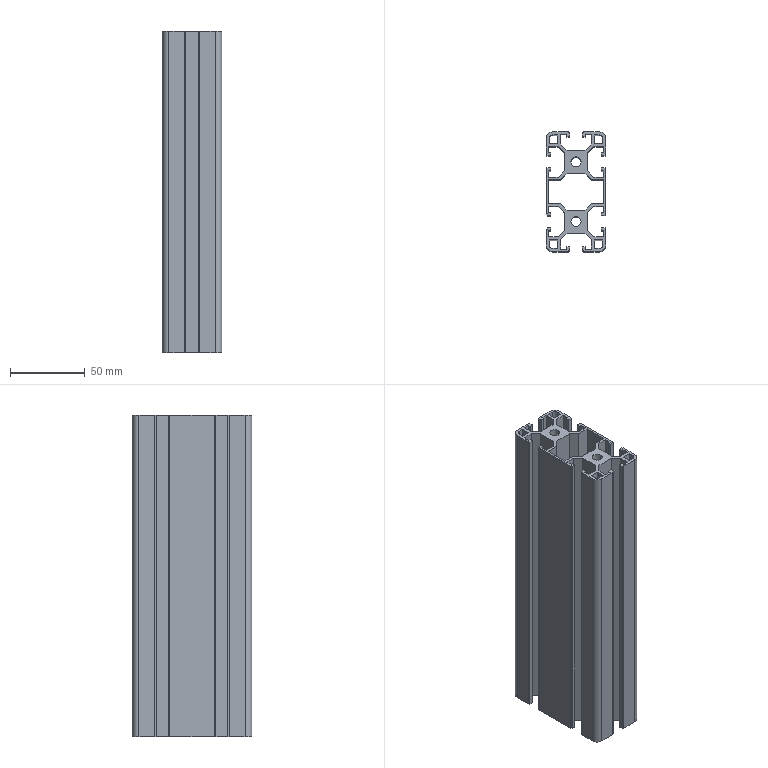Part | SolidWorks | features BaseBody 1 | 1 solid | 155 faces | box 40.002 x 80 x 215 mm | volume 211644 mm3 | plane 142 | cylinder 13 | commonest cylinder face diameters 9 x5 5 x4 6.8 x4